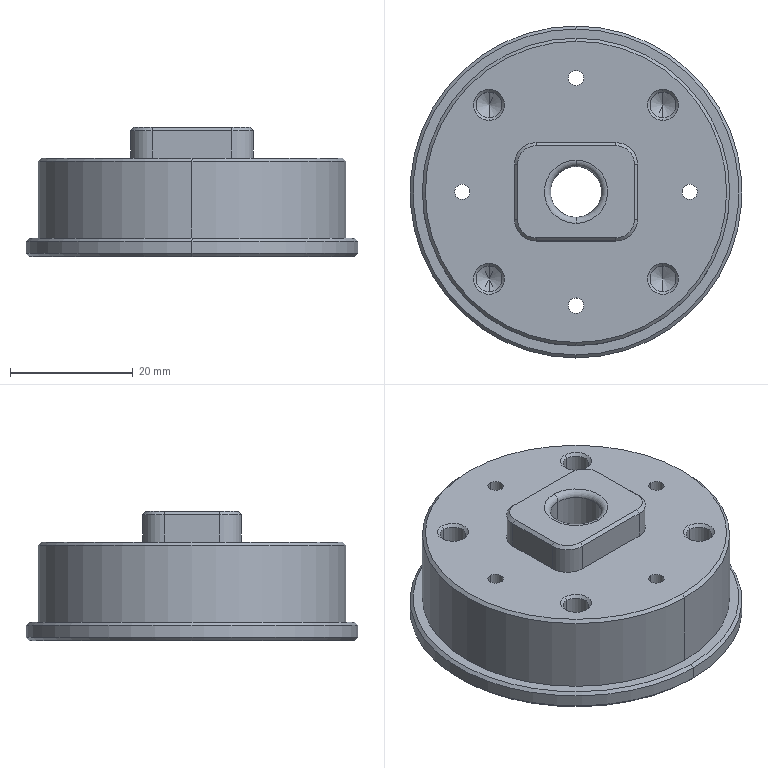NC program | NX | posted with a generic post | part box 54 x 54 x 21 mm
Whole program:
N10 G17 G21 G94 G90
(FLOOR_WALL , TOOL : D80)
N12 T19 M6
N14 G54
N16 G17 G0 G90 X-76. Y0. S6500 M3
N18 G43 Z30. H19
N20 Z3.
N22 G94 G1 Z0. F1500.
N24 X-73.
N26 X73.
N28 X76.
N30 Z3.
N32 G0 Z30.
N34 M5
(ADAPTIVE_MILLING , TOOL : D10)
N36 T15 M6
N38 G54
N40 G17 G0 G90 X-40.709 Y-0.765 S9500 M3
N42 G43 Z30. H15
N44 Z-1.85
N46 G94 G1 Z-4.85 F1000.
N48 X-38.815 Y-0.552 F3000.
N50 G3 X-38.053 Y-0.053 R1.025
N52 X-37.177 Y2.594 R8.702
N54 G2 X-35.179 Y10.978 R72.98
N56 X34.341 Y13.24 R36.833
N58 X36.684 Y3.031 R44.483
N60 X-36.628 Y-3.589 R36.806
N62 X-36.044 Y2.623 R30.952
N64 X-31.88 Y16.061 R45.576
N66 X32.87 Y13.815 R35.661
N68 X35.61 Y-2.194 R37.164
N70 X-35.193 Y-5.748 R35.666
N72 X-34.872 Y2.842 R30.272
N74 X-29.192 Y18.473 R40.634
N76 X31.454 Y14.189 R34.507
N78 X27.902 Y-20.344 R34.602
N80 X-33.752 Y-7.175 R34.498
N82 X-33.616 Y3.519 R30.666
N84 X-26.377 Y20.471 R37.474
N86 X-22.445 Y-24.709 R-33.375
N88 X-32.473 Y-7.489 R32.483
N90 X-32.17 Y5.048 R31.678
N92 X-21.41 Y24.087 R34.741
N94 X-29.968 Y-11.828 R-32.213
N96 X-31.408 Y2.804 R28.256
N98 X-21.955 Y21.98 R33.923
N100 X-28.182 Y-13.043 R-31.052
N102 X-30.17 Y3.213 R27.81
N104 X-19.228 Y22.888 R32.171
N106 X-26.395 Y-13.999 R-29.878
N108 X-29.045 Y2.869 R27.023
N110 X-17.559 Y22.719 R30.787
N112 X-24.076 Y-15.615 R-28.699
N114 X-27.897 Y2.569 R26.094
N116 X-14.238 Y23.552 R29.225
N118 X-22.926 Y-15.189 R-27.508
N120 X-26.568 Y3.363 R25.363
N122 X-11.058 Y23.884 R27.718
N124 X-21.36 Y-15.341 R-26.307
N126 X-25.287 Y3.705 R24.459
N128 X-9.086 Y23.407 R26.372
N130 X-19.352 Y-15.964 R-25.096
N132 X-24.039 Y3.791 R23.446
N134 X-7.07 Y22.818 R25.05
N136 X-17.363 Y-16.369 R-23.873
N138 X-22.703 Y4.185 R22.422
N140 X-4.927 Y22.106 R23.663
N142 X-15.927 Y-16.065 R-22.634
N144 X-21.292 Y4.726 R21.361
N146 X-2.197 Y21.281 R22.259
N148 X-14.178 Y-15.985 R-21.38
N150 X-19.904 Y5.029 R20.247
N152 X-1.273 Y20.081 R20.934
N154 X-12.358 Y-15.842 R-20.106
N156 X-18.428 Y5.45 R19.076
N158 X0.819 Y18.807 R19.526
N160 X-10.576 Y-15.537 R-18.808
N162 X-16.973 Y5.652 R17.859
N164 X1.353 Y17.452 R18.167
N166 X-8.225 Y-15.413 R-17.485
N168 X-15.375 Y6.035 R16.592
N170 X-13.659 Y9.346 R132.003
N172 X2.744 Y15.909 R17.086
N174 X10.823 Y11.95 R16.354
N176 X12.65 Y10.576 R8.667
N178 X15.009 Y6.481 R10.664
N180 X15.01 Y-5.926 R17.413
N182 X12.214 Y-10.995 R8.933
N184 X1.334 Y-16.081 R17.925
N186 X-10.542 Y-12.1 R15.823
N188 G1 X-11.26 Y-11.717
N190 X-11.346 Y-11.659
N192 G2 X-14.507 Y-7.76 R9.254
N194 X-15.15 Y2.504 R19.061
N196 X-14.969 Y6.237 R21.648
N198 G1 X-14.507 Y7.76
N200 X-14.096 Y8.56
N202 X-13.659 Y9.346
N204 X-13.126 Y10.004
N206 X-12.576 Y10.65
N208 G2 X-9.059 Y12.774 R9.748
N210 X-2.234 Y14.732 R25.451
N212 X6.625 Y13.168 R15.637
N214 G1 X8.237 Y12.969
N216 G2 X10.848 Y11.937 R9.097
N218 G3 X12.32 Y12.809 R1.002
N220 X12.01 Y13.568 Z-4.808 R1.184
N222 G1 X11.321 Y14.502 Z-4.75
N224 X10.767 Y15.261
N226 X10.196 Y16.008
N228 G3 X9.684 Y16.283 R1.05
N230 G1 X5.763 Y17.072
N232 X1.839 Y17.842
N234 G3 X-2.631 Y17.8 R14.477
N236 G1 X-8.596 Y16.853
N238 G3 X-9.269 Y16.423 R1.026
N240 G1 X-10.233 Y14.986
N242 X-10.608 Y14.437 Z-4.783
N244 X-10.962 Y13.875 Z-4.817
N246 G3 X-11.02 Y13.219 Z-4.85 R1.04
N248 X-9.76 Y12.507 R1.004
N250 G2 X-6.526 Y13.147 R10.071
N252 X-0.429 Y13.616 R33.625
N254 X2.8 Y13.15 R19.363
N256 X6.899 Y13.111 R63.021
N258 G3 X7.01 Y15.305 R-1.1
N260 G1 X-6.577 Y15.346
N262 G3 X-6.526 Y13.147 R-1.1
N264 G1 X-6.474 Y13.15
N266 X2.901
N268 X6.526 Y13.147
N270 X7.383 Y13.068
N272 X8.237 Y12.969
N274 X9.05 Y12.728
N276 X9.856 Y12.467
N278 X10.606 Y12.072
N280 X11.346 Y11.659
N282 X12.004 Y11.126
N284 X12.65 Y10.576
N286 X13.191 Y9.924
N288 X13.717 Y9.26
N290 X14.121 Y8.515
N292 X14.507 Y7.76
N294 G2 X15.15 Y4.474 R10.137
N296 G1 Y-4.474
N298 X15.147 Y-4.526
N300 X15. Y-6.019
N302 X14.969 Y-6.237
N304 X14.728 Y-7.05
N306 X14.467 Y-7.856
N308 X14.072 Y-8.606
N310 X13.659 Y-9.346
N312 X13.126 Y-10.004
N314 X12.576 Y-10.65
N316 G2 X9.172 Y-12.717 R9.474
N318 X2.844 Y-14.626 R29.145
N320 X-6.515 Y-13.18 R15.434
N322 G3 X-8.237 Y-12.969 R35.086
N324 G1 X-9.76 Y-12.507
N326 X-9.856 Y-12.467
N328 X-10.628 Y-12.054
N330 G3 X-12.099 Y-12.923 R1.002
N332 X-11.79 Y-13.685 Z-4.808 R1.182
N334 G1 X-11.102 Y-14.617 Z-4.75
N336 X-10.547 Y-15.378
N338 X-9.976 Y-16.126
N340 G3 X-9.463 Y-16.401 R1.05
N342 G1 X-6.34 Y-17.031
N344 X-3.212 Y-17.638
N346 G3 X3.492 Y-17.661 R21.206
N348 G1 X8.596 Y-16.853
N350 G3 X9.27 Y-16.423 R1.026
N352 G1 X10.233 Y-14.987
N354 X10.608 Y-14.437 Z-4.783
N356 X10.962 Y-13.875 Z-4.817
N358 G3 X11.02 Y-13.22 Z-4.85 R1.04
N360 X9.76 Y-12.507 R1.004
N362 G2 X6.402 Y-13.161 R10.665
N364 X0.302 Y-13.591 R32.643
N366 X-2.687 Y-13.15 R19.438
N368 G1 X-6.775 Y-13.123
N370 G3 X-6.885 Y-15.318 R-1.1
N372 G1 X6.578 Y-15.346
N374 G3 X6.526 Y-13.147 R-1.1
N376 G1 X6.474 Y-13.15
N378 X-2.776
N380 X-6.526 Y-13.147
N382 X-7.383 Y-13.068
N384 X-8.237 Y-12.969
N386 X-9.05 Y-12.728
N388 X-9.856 Y-12.467
N390 X-10.606 Y-12.072
N392 X-11.346 Y-11.659
N394 X-12.004 Y-11.126
N396 X-12.65 Y-10.576
N398 X-13.191 Y-9.924
N400 X-13.717 Y-9.26
N402 X-14.121 Y-8.515
N404 X-14.507 Y-7.76
N406 X-14.969 Y-6.237
N408 X-14.989 Y-6.136
N410 X-15.147 Y-4.526
N412 X-15.15 Y-4.474
N414 Y2.526
N416 G3 X-15.682 Y3.416 R1.021
N418 G1 X-17.65 Y4.474
N420 Z-1.85
N422 G0 Z30.
N424 X-40.701 Y0.196
N426 Z-14.85
N428 G1 Z-17.85 F1000.
N430 X-39.23 Y-0.263 F3000.
N432 G3 X-38.054 Y0.196 R1.017
N434 X-37.132 Y2.959 R9.118
N436 G2 X-34.745 Y12.274 R66.025
N438 X34.338 Y13.25 R36.83
N440 X36.704 Y2.792 R43.918
N442 X-36.659 Y-3.229 R36.805
N444 X-35.96 Y3.222 R32.784
N446 X-31.606 Y16.599 R45.295
N448 X32.909 Y13.721 R35.667
N450 X35.513 Y-3.417 R36.906
N452 X-35.264 Y-5.281 R35.663
N454 X-34.788 Y3.427 R31.004
N456 X-28.874 Y18.969 R40.318
N458 X34.35 Y3.273 R34.529
N460 X-33.799 Y-6.97 R34.506
N462 X-33.651 Y3.353 R30.275
N464 X-26.639 Y20.141 R37.772
N466 X-1.943 Y-33.326 R-33.38
N468 X-32.339 Y-8.15 R33.25
N470 X-32.424 Y3.77 R29.972
N472 X-23.512 Y22.046 R35.376
N474 X-22.345 Y-23.217 R-32.218
N476 X-31.239 Y-7.58 R30.96
N478 X-30.84 Y5.808 R31.229
N480 X-18.301 Y25.095 R32.979
N482 X-28.556 Y-12.194 R-31.049
N484 X-30.171 Y3.262 R27.83
N486 X-28.806 Y8.74 R35.89
N488 G1 X-28.368 Y10.206
N490 X-28.348 Y10.262
N492 X-27.039 Y13.336
N494 X-27.012 Y13.389
N496 X-25.391 Y16.255
N498 X-25.359 Y16.305
N500 X-23.429 Y18.974
N502 X-23.391 Y19.02
N504 X-21.177 Y21.458
N506 X-21.135 Y21.5
N508 X-18.663 Y23.677
N510 X-18.617 Y23.713
N512 X-15.919 Y25.603
N514 X-15.869 Y25.634
N516 X-12.978 Y27.212
N518 X-12.925 Y27.237
N520 X-9.876 Y28.485
N522 X-9.82 Y28.504
N524 X-6.652 Y29.405
N526 X-6.595 Y29.418
N528 X-3.346 Y29.962
N530 X-3.287 Y29.969
N532 X0.03 Y30.15
N534 X3.343 Y29.962
N536 X3.401 Y29.956
N538 X6.643 Y29.407
N540 X6.7 Y29.394
N542 X9.861 Y28.49
N544 X9.917 Y28.471
N546 X12.958 Y27.222
N548 X13.011 Y27.196
N550 X15.895 Y25.618
N552 X15.945 Y25.587
N554 X18.637 Y23.698
N556 X18.683 Y23.662
N558 X21.148 Y21.487
N560 X21.19 Y21.445
N562 X23.399 Y19.01
N564 X23.436 Y18.965
N566 X25.362 Y16.3
N568 X25.394 Y16.25
N570 X27.012 Y13.389
N572 X27.039 Y13.336
N574 X28.347 Y10.266
N576 X28.367 Y10.209
N578 X29.322 Y7.012
N580 X29.335 Y6.954
N582 X29.924 Y3.669
N584 X29.931 Y3.61
N586 X30.148 Y0.267
N588 X30.149 Y0.246
N590 X29.987 Y-3.113
N592 X29.981 Y-3.172
N594 X29.447 Y-6.466
N596 X29.434 Y-6.524
N598 X28.533 Y-9.737
N600 X28.513 Y-9.794
N602 X27.256 Y-12.885
N604 X27.231 Y-12.939
N606 X25.634 Y-15.869
N608 X25.603 Y-15.919
N610 X23.687 Y-18.651
N612 X23.65 Y-18.698
N614 X21.438 Y-21.197
N616 X21.396 Y-21.24
N618 X18.918 Y-23.474
N620 X18.871 Y-23.512
N622 X16.158 Y-25.453
N624 X16.107 Y-25.485
N626 X13.192 Y-27.109
N628 X13.138 Y-27.135
N630 X10.059 Y-28.421
N632 X10.003 Y-28.441
N634 X6.798 Y-29.372
N636 X6.74 Y-29.385
N638 X3.452 Y-29.95
N640 X3.392 Y-29.957
N642 X0.03 Y-30.15
N644 X-3.334 Y-29.963
N646 X-3.394 Y-29.957
N648 X-6.687 Y-29.397
N650 X-6.745 Y-29.384
N652 X-9.954 Y-28.458
N654 X-10.011 Y-28.438
N656 X-13.095 Y-27.156
N658 X-13.149 Y-27.13
N660 X-16.069 Y-25.509
N662 X-16.12 Y-25.477
N664 X-18.839 Y-23.537
N666 X-18.886 Y-23.5
N668 X-21.37 Y-21.266
N670 X-21.412 Y-21.224
N672 X-23.628 Y-18.725
N674 X-23.665 Y-18.678
N676 X-25.586 Y-15.946
N678 X-25.618 Y-15.895
N680 X-27.219 Y-12.963
N682 X-27.245 Y-12.909
N684 X-28.505 Y-9.816
N686 X-28.525 Y-9.76
N688 X-29.429 Y-6.544
N690 X-29.442 Y-6.486
N692 X-29.979 Y-3.189
N694 X-29.985 Y-3.13
N696 X-30.149 Y0.232
N698 X-30.148 Y0.254
N700 X-29.933 Y3.6
N702 X-29.925 Y3.659
N704 X-29.337 Y6.947
N706 X-29.323 Y7.005
N708 X-28.787 Y8.802
N710 G3 X-29.612 Y10.091 R1.014
N712 G1 X-30.954 Y10.282
N714 Z-14.85
N716 G0 Z30.
N718 X-40.701 Y1.071
N720 Z-18.
N722 G1 Z-21. F1000.
N724 X-39.861 Y0.832 F3000.
N726 X-39.014 Y0.617
N728 G3 X-38.054 Y1.071 R1.021
N730 X-37.149 Y3.443 R7.669
N732 G2 X-34.848 Y12.009 R79.795
N734 X34.105 Y13.869 R36.854
N736 X36.711 Y2.703 R43.491
N738 X2.721 Y-36.725 R36.81
N740 X-36.731 Y-2.395 R36.81
N742 X-35.832 Y4.283 R34.004
N744 X-31.217 Y17.309 R44.711
N746 X32.929 Y13.665 R35.657
N748 X35.468 Y-3.849 R36.801
N750 X-35.364 Y-4.604 R35.668
N752 X-34.754 Y3.97 R30.499
N754 X-28.788 Y19.101 R40.841
N756 X31.65 Y13.733 R34.506
N758 X-33.951 Y-6.204 R-34.511
N760 X-33.525 Y4.358 R30.471
N762 X-25.78 Y21.22 R37.629
N764 X-18.885 Y-27.528 R-33.376
N766 X-32.592 Y-7.052 R32.952
N768 X-32.18 Y5.232 R30.753
N770 X-21.936 Y23.615 R35.007
N772 X-30.501 Y-10.383 R-32.215
N774 X-31.636 Y-5.718 R41.55
N776 G1 X-32.062 Y-2.361
N778 X-32.066 Y-2.305
N780 X-32.131 Y1.091
N782 X-32.129 Y1.131
N784 X-31.831 Y4.507
N786 X-31.823 Y4.563
N788 X-31.167 Y7.883
N790 X-31.153 Y7.938
N792 X-30.146 Y11.169
N794 X-30.126 Y11.222
N796 X-28.78 Y14.326
N798 X-28.754 Y14.378
N800 X-27.018 Y17.423
N802 X-26.986 Y17.472
N804 X-24.924 Y20.306
N806 X-24.886 Y20.351
N808 X-22.523 Y22.94
N810 X-22.481 Y22.981
N812 X-19.846 Y25.291
N814 X-19.8 Y25.328
N816 X-16.925 Y27.332
N818 X-16.875 Y27.363
N820 X-13.796 Y29.038
N822 X-13.743 Y29.063
N824 X-10.498 Y30.386
N826 X-10.442 Y30.405
N828 X-7.071 Y31.361
N830 X-7.013 Y31.374
N832 X-3.556 Y31.951
N834 X-3.498 Y31.958
N836 X0.03 Y32.15
N838 X3.553 Y31.951
N840 X3.612 Y31.945
N842 X7.062 Y31.363
N844 X7.119 Y31.35
N846 X10.483 Y30.391
N848 X10.539 Y30.372
N850 X13.777 Y29.047
N852 X13.83 Y29.022
N854 X16.902 Y27.347
N856 X16.951 Y27.316
N858 X19.819 Y25.312
N860 X19.866 Y25.276
N862 X22.495 Y22.968
N864 X22.536 Y22.927
N866 X24.894 Y20.342
N868 X24.931 Y20.296
N870 X26.989 Y17.467
N872 X27.021 Y17.418
N874 X28.754 Y14.378
N876 X28.78 Y14.326
N878 X30.125 Y11.225
N880 X30.145 Y11.172
N882 X31.151 Y7.944
N884 X31.165 Y7.889
N886 X31.822 Y4.573
N888 X31.83 Y4.516
N890 X32.128 Y1.144
N892 X32.13 Y1.104
N894 X32.067 Y-2.288
N896 X32.063 Y-2.345
N898 X31.639 Y-5.699
N900 X31.629 Y-5.755
N902 X30.85 Y-9.045
N904 X30.834 Y-9.099
N906 X29.708 Y-12.287
N908 X29.686 Y-12.34
N910 X28.226 Y-15.389
N912 X28.199 Y-15.439
N914 X26.421 Y-18.315
N916 X26.389 Y-18.362
N918 X24.315 Y-21.031
N920 X24.278 Y-21.074
N922 X21.93 Y-23.507
N924 X21.889 Y-23.546
N926 X19.295 Y-25.715
N928 X19.249 Y-25.749
N930 X16.439 Y-27.628
N932 X16.39 Y-27.657
N934 X13.395 Y-29.225
N936 X13.343 Y-29.249
N938 X10.198 Y-30.488
N940 X10.144 Y-30.506
N942 X6.884 Y-31.403
N944 X6.829 Y-31.415
N946 X3.492 Y-31.958
N948 X3.435 Y-31.964
N950 X0.03 Y-32.15
N952 X-3.377 Y-31.971
N954 X-3.433 Y-31.965
N956 X-6.774 Y-31.427
N958 X-6.83 Y-31.415
N960 X-10.094 Y-30.523
N962 X-10.148 Y-30.505
N964 X-13.299 Y-29.269
N966 X-13.35 Y-29.245
N968 X-16.351 Y-27.68
N970 X-16.4 Y-27.651
N972 X-19.215 Y-25.774
N974 X-19.261 Y-25.74
N976 X-21.86 Y-23.573
N978 X-21.902 Y-23.534
N980 X-24.254 Y-21.101
N982 X-24.291 Y-21.058
N984 X-26.37 Y-18.388
N986 X-26.403 Y-18.342
N988 X-28.185 Y-15.465
N990 X-28.212 Y-15.415
N992 X-29.676 Y-12.364
N994 X-29.698 Y-12.311
N996 X-30.827 Y-9.121
N998 X-30.843 Y-9.067
N1000 X-31.508 Y-6.27
N1002 G3 X-32.472 Y-5.493 R1.017
N1004 G1 X-34.186 Y-5.462
N1006 Z-18.
N1008 G0 Z30.
N1010 M5
(ZLEVEL_PROFILE_COPY_1_COPY_COPY_1 , TOOL : D10JING)
N1012 T14 M6
N1014 G54
N1016 G17 G0 G90 X-33.957 Y-1.707 S9500 M3
N1018 G43 Z30. H14
N1020 Z-20.
N1022 G94 G1 Z-21. F1000.
N1024 X-32.5 Y-0.866
N1026 G3 X-32. Y0. R1.
N1028 G2 X0. Y32. R32. F1200.
N1030 X-32. Y0. R-32.
N1032 G3 X-32.5 Y0.866 R1.
N1034 G1 X-33.957 Y1.707
N1036 Z-20.
N1038 G0 Z30.
(FLOOR_WALL_1_COPY , TOOL : D10JING)
N1040 X0. Y-32.5
N1042 Z-2.
N1044 G1 Z-5. F1250.
N1046 Y-29.5
N1048 G2 X-29.5 Y0. R29.5
N1050 X0. Y-29.5 R-29.5
N1052 G1 Y-24.5
N1054 G2 X-24.5 Y0. R24.5
N1056 X0. Y-24.5 R-24.5
N1058 G1 Y-19.5
N1060 G2 X4.473 Y18.98 R-19.5
N1062 G1 X3.441 Y14.6
N1064 X-3.441
N1066 G2 X3.441 Y14.6 R15.
N1068 G1 X4.473 Y18.98
N1070 G2 X0. Y-19.5 R19.5
N1072 G1 Y-15.
N1074 G2 X-3.441 Y-14.6 R15.
N1076 G1 X3.441
N1078 Y-13.6
N1080 X-6.5
N1082 G2 X-15.6 Y-4.5 R9.1
N1084 G1 Y4.5
N1086 G2 X-6.5 Y13.6 R9.1
N1088 G1 X6.5
N1090 G2 X15.6 Y4.5 R9.1
N1092 G1 Y-4.5
N1094 G2 X6.5 Y-13.6 R9.1
N1096 G1 X3.441
N1098 Y-14.6
N1100 G2 X0. Y-15. R15.
N1102 G1 Y-16.6
N1104 Y-13.1
N1106 X-6.5
N1108 G2 X-15.1 Y-4.5 R8.6
N1110 G1 Y4.5
N1112 G2 X-6.5 Y13.1 R8.6
N1114 G1 X6.5
N1116 G2 X15.1 Y4.5 R8.6
N1118 G1 Y-4.5
N1120 G2 X6.5 Y-13.1 R8.6
N1122 G1 X0.
N1124 Y-16.6
N1126 Z-2.
N1128 G0 Z30.
N1130 Y-33.6
N1132 Z-15.
N1134 G1 Z-18.
N1136 Y-30.6
N1138 G2 X-30.6 Y0. R30.6
N1140 X0. Y-30.6 R-30.6
N1142 G1 Y-34.5
N1144 Y-30.1
N1146 G2 X-30.1 Y0. R30.1
N1148 X0. Y-30.1 R-30.1
N1150 G1 Y-33.6
N1152 Z-15.
N1154 G0 Z30.
N1156 M5
(DRILLING , TOOL : D6A45)
N1158 T01 M6
N1160 G54
N1162 G17 G0 G90 X0. Y0. S5000 M3
N1164 G43 Z30. H1
N1166 G94 G81 G98 Z-1.35 F350. R3.
N1168 Y-18.5 Z-6.35 R-2.
N1170 X14.142 Y-14.142
N1172 X18.5 Y0.
N1174 X14.142 Y14.142
N1176 X0. Y18.5
N1178 X-14.142 Y14.142
N1180 X-18.5 Y0.
N1182 X-14.142 Y-14.142
N1184 G80
N1186 G0 X-14.142 Y-14.142 Z30.
N1188 M5
(DRILLING_COPY , TOOL : 2.5ZT)
N1190 T02 M6
N1192 G54
N1194 G17 G0 G90 X0. Y18.5 S2000 M3
N1196 G43 Z30. H2
N1198 G94 G83 G98 Z-16.5 F120. Q2. R-2.
N1200 X-18.5 Y0.
N1202 X0. Y-18.5
N1204 X18.5 Y0.
N1206 G80
N1208 G0 X18.5 Y0. Z30.
N1210 M5
(DRILLING_COPY_COPY , TOOL : 4.2ZT)
N1212 T04 M6
N1214 G54
N1216 G17 G0 G90 X14.142 Y-14.142 S2000 M3
N1218 G43 Z30. H4
N1220 G94 G83 G98 Z-20.262 F250. Q2. R-2.
N1222 X-14.142
N1224 Y14.142
N1226 X14.142
N1228 G80
N1230 G0 X14.142 Y14.142 Z30.
(DRILLING_COPY_COPY_COPY , TOOL : 4.2ZT)
N1232 X0. Y0.
N1234 G83 Z-21.262 F250. Q2. R3.
N1236 G80
N1238 G0 X0. Y0. Z30.
N1240 M5
(HOLE_MILLING , TOOL : D6)
N1242 T12 M6
N1244 G54
N1246 G17 G0 G90 X0. Y0. S9500 M3
N1248 G43 Z30. H12
N1250 Z0.5
N1252 G94 G3 X0.575 Y-0.575 R0.575 F1200.
N1254 X1.15 Y0. R0.575
N1256 X1.15 Y0. Z0. I-1.15 J0.
N1258 X1.15 Y0. Z-0.5 I-1.15 J0.
N1260 X1.15 Y0. Z-1. I-1.15 J0.
N1262 X1.15 Y0. Z-1.5 I-1.15 J0.
N1264 X1.15 Y0. Z-2. I-1.15 J0.
N1266 X1.15 Y0. Z-2.5 I-1.15 J0.
N1268 X1.15 Y0. Z-3. I-1.15 J0.
N1270 X1.15 Y0. Z-3.5 I-1.15 J0.
N1272 X1.15 Y0. Z-4. I-1.15 J0.
N1274 X1.15 Y0. Z-4.5 I-1.15 J0.
N1276 X1.15 Y0. Z-5. I-1.15 J0.
N1278 X1.15 Y0. Z-5.5 I-1.15 J0.
N1280 X1.15 Y0. Z-6. I-1.15 J0.
N1282 X1.15 Y0. Z-6.5 I-1.15 J0.
N1284 X1.15 Y0. Z-7. I-1.15 J0.
N1286 X1.15 Y0. Z-7.5 I-1.15 J0.
N1288 X1.15 Y0. Z-8. I-1.15 J0.
N1290 X1.15 Y0. Z-8.5 I-1.15 J0.
N1292 X1.15 Y0. Z-9. I-1.15 J0.
N1294 X1.15 Y0. Z-9.5 I-1.15 J0.
N1296 X1.15 Y0. Z-10. I-1.15 J0.
N1298 X1.15 Y0. Z-10.5 I-1.15 J0.
N1300 X1.15 Y0. Z-11. I-1.15 J0.
N1302 X1.15 Y0. Z-11.5 I-1.15 J0.
N1304 X1.15 Y0. Z-12. I-1.15 J0.
N1306 X1.15 Y0. Z-12.5 I-1.15 J0.
N1308 X1.15 Y0. Z-13. I-1.15 J0.
N1310 X1.15 Y0. Z-13.5 I-1.15 J0.
N1312 X1.15 Y0. Z-14. I-1.15 J0.
N1314 X1.15 Y0. Z-14.5 I-1.15 J0.
N1316 X1.15 Y0. Z-15. I-1.15 J0.
N1318 X1.15 Y0. Z-15.5 I-1.15 J0.
N1320 X1.15 Y0. Z-16. I-1.15 J0.
N1322 X1.15 Y0. Z-16.5 I-1.15 J0.
N1324 X1.15 Y0. Z-17. I-1.15 J0.
N1326 X1.15 Y0. Z-17.5 I-1.15 J0.
N1328 X1.15 Y0. Z-18. I-1.15 J0.
N1330 X1.15 Y0. Z-18.5 I-1.15 J0.
N1332 X1.15 Y0. Z-19. I-1.15 J0.
N1334 X1.15 Y0. Z-19.5 I-1.15 J0.
N1336 X0. Y1.15 R1.15
N1338 X1.15 Y0. R-1.15
N1340 X0.575 Y0.575 R0.575
N1342 X0. Y0. R0.575
N1344 G0 Z30.
N1346 M5
(ZLEVEL_PROFILE_1 , TOOL : D4R0.5)
N1348 T17 M6
N1350 G54
N1352 G17 G0 G90 X-2.55 Y0.756 S9500 M3
N1354 G43 Z30. H17
N1356 Z1.488
N1358 G94 G1 Z-0.012 F2500.
N1360 X-3.26 Y0.346
N1362 G3 X-3.46 Y0. R0.4
N1364 X0. Y-3.46 R3.46
N1366 X-3.46 Y0. R-3.46
N1368 G1 X-3.399 Z-0.021
N1370 X-3.35 Z-0.03
N1372 G2 X0. Y3.35 R3.35
N1374 X-3.35 Y0. R-3.35
N1376 G1 X-3.294 Z-0.043
N1378 X-3.247 Z-0.055
N1380 G3 X0. Y-3.247 R3.247
N1382 X-3.247 Y0. R-3.247
N1384 G1 X-3.195 Z-0.071
N1386 X-3.148 Z-0.086
N1388 G2 X0. Y3.148 R3.148
N1390 X-3.148 Y0. R-3.148
N1392 G1 X-3.098 Z-0.105
N1394 X-3.053 Z-0.124
N1396 G3 X0. Y-3.053 R3.053
N1398 X-3.053 Y0. R-3.053
N1400 G1 X-3.005 Z-0.146
N1402 X-2.962 Z-0.167
N1404 G2 X0. Y2.962 R2.962
N1406 X-2.962 Y0. R-2.962
N1408 G1 X-2.916 Z-0.192
N1410 X-2.873 Z-0.217
N1412 G3 X0. Y-2.873 R2.873
N1414 X-2.873 Y0. R-2.873
N1416 G1 X-2.829 Z-0.244
N1418 X-2.789 Z-0.272
N1420 G2 X0. Y2.789 R2.789
N1422 X-2.789 Y0. R-2.789
N1424 G1 X-2.747 Z-0.302
N1426 X-2.708 Z-0.332
N1428 G3 X0. Y-2.708 R2.708
N1430 X-2.708 Y0. R-2.708
N1432 G1 X-2.669 Z-0.365
N1434 X-2.632 Z-0.398
N1436 G2 X0. Y2.632 R2.632
N1438 X-2.632 Y0. R-2.632
N1440 G1 X-2.595 Z-0.433
N1442 X-2.561 Z-0.469
N1444 G3 X0. Y-2.561 R2.561
N1446 X-2.561 Y0. R-2.561
N1448 G1 X-2.526 Z-0.506
N1450 X-2.494 Z-0.544
N1452 G2 X0. Y2.494 R2.494
N1454 X-2.494 Y0. R-2.494
N1456 G1 X-2.462 Z-0.584
N1458 X-2.433 Z-0.623
N1460 G3 X0. Y-2.433 R2.433
N1462 X-2.433 Y0. R-2.433
N1464 G1 X-2.404 Z-0.665
N1466 X-2.377 Z-0.707
N1468 G2 X0. Y2.377 R2.377
N1470 X-2.377 Y0. R-2.377
N1472 G1 X-2.351 Z-0.75
N1474 X-2.327 Z-0.793
N1476 G3 X0. Y-2.327 R2.327
N1478 X-2.327 Y0. R-2.327
N1480 G1 X-2.304 Z-0.838
N1482 X-2.283 Z-0.883
N1484 G2 X0. Y2.283 R2.283
N1486 X-2.283 Y0. R-2.283
N1488 G1 X-2.263 Z-0.929
N1490 X-2.245 Z-0.976
N1492 G3 X0. Y-2.245 R2.245
N1494 X-2.245 Y0. R-2.245
N1496 G1 X-2.228 Z-1.023
N1498 X-2.213 Z-1.071
N1500 G2 X0. Y2.213 R2.213
N1502 X-2.213 Y0. R-2.213
N1504 G1 X-2.199 Z-1.119
N1506 X-2.187 Z-1.167
N1508 G3 X0. Y-2.187 R2.187
N1510 X-2.187 Y0. R-2.187
N1512 G1 X-2.178 Z-1.209
N1514 X-2.171 Z-1.251
N1516 G2 X0. Y2.171 R2.171
N1518 X-2.171 Y0. R-2.171
N1520 G1 X-2.164 Z-1.292
N1522 X-2.159 Z-1.334
N1524 G3 X0. Y-2.159 R2.159
N1526 X-2.159 Y0. R-2.159
N1528 G1 X-2.152 Z-1.417
N1530 G2 X-2.088 Y0.52 R2.152
N1532 G1 X-2.077 Y0.564
N1534 G2 X-1.275 Y1.734 R2.152
N1536 G1 X-1.128 Y1.833
N1538 G2 X2.085 Y-0.535 R2.152
N1540 G1 X2.077 Y-0.564
N1542 G2 X1.265 Y-1.741 R2.152
N1544 G1 X1.237 Y-1.761
N1546 X1.205 Y-1.784
N1548 X1.128 Y-1.833
N1550 G2 X0.564 Y-2.077 R2.152
N1552 G1 X0.282 Y-2.134
N1554 G2 X-1.295 Y-1.719 R2.152
N1556 G1 X-1.334 Y-1.689
N1558 G2 X-2.152 Y0. R2.152
N1560 G1 X-2.15 Z-1.5
N1562 G3 X0. Y-2.15 R2.15
N1564 X-2.15 Y0. R-2.15
N1566 X-1.95 Y-0.346 R0.4
N1568 G1 X-1.022 Y-0.882
N1570 Z0.
N1572 G0 Z30.
N1574 M5
(PLANAR_MILL_COPY_COPY_COPY_COPY_COPY_COPY_1 , TOOL : D6A45)
N1576 T01 M6
N1578 G54
N1580 G17 G0 G90 X0.866 Y-9.5 S9500 M3
N1582 G43 Z30. H1
N1584 Z0.
N1586 G94 G1 Z-1.5 F1250.
N1588 G3 X0. Y-9. R1.
N1590 G1 X-6.5
N1592 G2 X-11. Y-4.5 R4.5
N1594 G1 Y4.5
N1596 G2 X-6.5 Y9. R4.5
N1598 G1 X6.5
N1600 G2 X11. Y4.5 R4.5
N1602 G1 Y-4.5
N1604 G2 X6.5 Y-9. R4.5
N1606 G1 X0.
N1608 G3 X-0.866 Y-9.5 R1.
N1610 G1 Z0.
N1612 G0 Z30.
(PLANAR_MILL_COPY_COPY_COPY_COPY_COPY_COPY_1_COPY , TOOL : D6A45)
N1614 X13.276 Y13.617
N1616 Z-5.
N1618 G1 Z-6.5
N1620 G3 X14.142 Y13.117 R1.
N1622 X15.167 Y14.142 R1.025
N1624 X14.142 Y13.117 R-1.025
N1626 X15.008 Y13.617 R1.
N1628 G1 Z-5.
N1630 G0 Z30.
N1632 X13.276 Y-14.667
N1634 Z-5.
N1636 G1 Z-6.5
N1638 G3 X14.142 Y-15.167 R1.
N1640 X15.167 Y-14.142 R1.025
N1642 X14.142 Y-15.167 R-1.025
N1644 X15.008 Y-14.667 R1.
N1646 G1 Z-5.
N1648 G0 Z30.
N1650 X0.866 Y-26.5
N1652 Z-5.
N1654 G1 Z-6.5
N1656 G3 X0. Y-26. R1.
N1658 G2 X-26. Y0. R26.
N1660 X0. Y-26. R-26.
N1662 G3 X-0.866 Y-26.5 R1.
N1664 G1 Z-5.
N1666 G0 Z30.
N1668 X-15.008 Y-14.667
N1670 Z-5.
N1672 G1 Z-6.5
N1674 G3 X-14.142 Y-15.167 R1.
N1676 X-13.117 Y-14.142 R1.025
N1678 X-14.142 Y-15.167 R-1.025
N1680 X-13.276 Y-14.667 R1.
N1682 G1 Z-5.
N1684 G0 Z30.
N1686 X-15.008 Y13.617
N1688 Z-5.
N1690 G1 Z-6.5
N1692 G3 X-14.142 Y13.117 R1.
N1694 X-13.117 Y14.142 R1.025
N1696 X-14.142 Y13.117 R-1.025
N1698 X-13.276 Y13.617 R1.
N1700 G1 Z-5.
N1702 G0 Z30.
N1704 M5
(CUTTERCOMP14 , TOOL : D10JING)
N1706 T14 M6
N1708 G54
N1710 G17 G0 G90 X-31.123 Y-1.177 S9500 M3
N1712 G43 Z30. H14
N1714 Z-17.
N1716 G94 G1 Z-18. F1250.
N1718 G41 X-31.029 Y-1.143 D14
N1720 X-30.55 Y-0.866
N1722 G3 X-30.05 Y0. R1.
N1724 G2 X0. Y30.05 R30.05
N1726 X-30.05 Y0. R-30.05
N1728 G3 X-30.55 Y0.866 R1.
N1730 G1 X-31.029 Y1.143
N1732 G40
N1734 X-31.123 Y1.177
N1736 Z-17.
N1738 G0 Z30.
N1740 M5
(CUTTERCOMP14_COPY , TOOL : D6)
N1742 T12 M6
N1744 G54
N1746 G17 G0 G90 X-7.427 Y12.091 S9500 M3
N1748 G43 Z30. H12
N1750 Z-4.
N1752 G94 G1 Z-5. F1250.
N1754 G41 X-7.393 Y11.997 D12
N1756 X-7.02 Y11.35
N1758 G3 X-6.5 Y11.05 R0.6
N1760 G1 X6.5
N1762 G2 X13.05 Y4.5 R6.55
N1764 G1 Y-4.5
N1766 G2 X6.5 Y-11.05 R6.55
N1768 G1 X-6.5
N1770 G2 X-13.05 Y-4.5 R6.55
N1772 G1 Y4.5
N1774 G2 X-6.5 Y11.05 R6.55
N1776 G3 X-5.98 Y11.35 R0.6
N1778 G1 X-5.576 Y12.05
N1780 G40
N1782 X-5.542 Y12.144
N1784 Z-4.
N1786 G0 Z30.
N1788 M5
N1790 M2